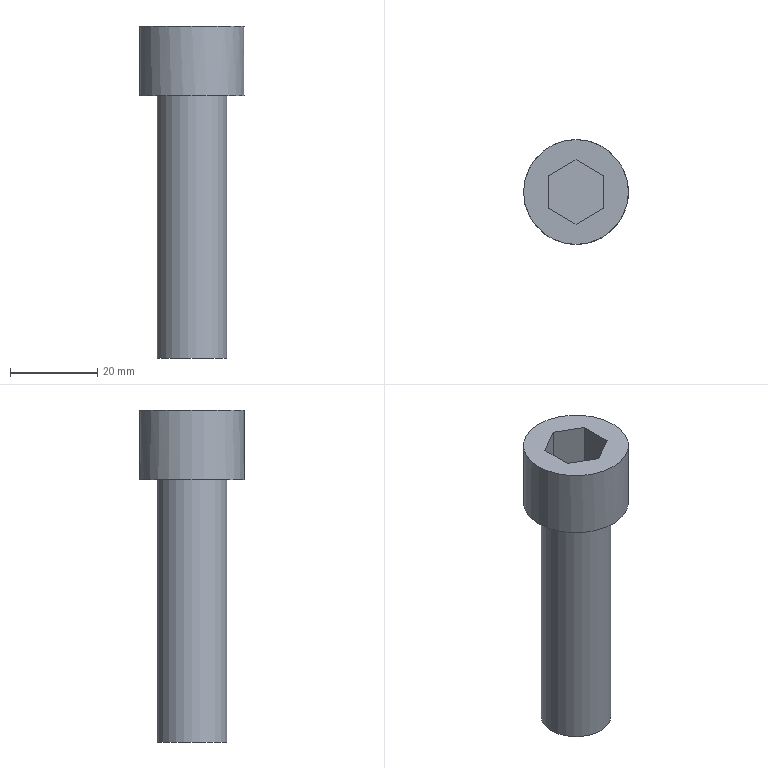Part | NX | features solid 2 | 1 solid | 12 faces | box 24 x 24 x 76 mm | volume 17940 mm3 | plane 10 | cylinder 2 | commonest cylinder face diameters 16 x1 24 x1
STEP:
#1=CARTESIAN_POINT('',(63.4,701.71,-169.));
#2=VERTEX_POINT('',#1);
#3=CARTESIAN_POINT('',(57.,698.015,-169.));
#4=VERTEX_POINT('',#3);
#5=CARTESIAN_POINT('',(60.2,699.862,-169.));
#6=DIRECTION('',(-0.866,-0.5,0.));
#7=VECTOR('',#6,1000.);
#8=LINE('',#5,#7);
#9=EDGE_CURVE('',#2,#4,#8,.T.);
#10=ORIENTED_EDGE('',*,*,#9,.T.);
#11=CARTESIAN_POINT('',(50.6,701.71,-169.));
#12=VERTEX_POINT('',#11);
#13=CARTESIAN_POINT('',(53.8,699.862,-169.));
#14=DIRECTION('',(-0.866,0.5,0.));
#15=VECTOR('',#14,1000.);
#16=LINE('',#13,#15);
#17=EDGE_CURVE('',#4,#12,#16,.T.);
#18=ORIENTED_EDGE('',*,*,#17,.T.);
#19=CARTESIAN_POINT('',(50.6,709.1,-169.));
#20=VERTEX_POINT('',#19);
#21=CARTESIAN_POINT('',(50.6,705.405,-169.));
#22=DIRECTION('',(0.,1.,0.));
#23=VECTOR('',#22,1000.);
#24=LINE('',#21,#23);
#25=EDGE_CURVE('',#12,#20,#24,.T.);
#26=ORIENTED_EDGE('',*,*,#25,.T.);
#27=CARTESIAN_POINT('',(57.,712.795,-169.));
#28=VERTEX_POINT('',#27);
#29=CARTESIAN_POINT('',(53.8,710.947,-169.));
#30=DIRECTION('',(0.866,0.5,0.));
#31=VECTOR('',#30,1000.);
#32=LINE('',#29,#31);
#33=EDGE_CURVE('',#20,#28,#32,.T.);
#34=ORIENTED_EDGE('',*,*,#33,.T.);
#35=CARTESIAN_POINT('',(63.4,709.1,-169.));
#36=VERTEX_POINT('',#35);
#37=CARTESIAN_POINT('',(60.2,710.947,-169.));
#38=DIRECTION('',(0.866,-0.5,0.));
#39=VECTOR('',#38,1000.);
#40=LINE('',#37,#39);
#41=EDGE_CURVE('',#28,#36,#40,.T.);
#42=ORIENTED_EDGE('',*,*,#41,.T.);
#43=CARTESIAN_POINT('',(63.4,705.405,-169.));
#44=DIRECTION('',(0.,-1.,0.));
#45=VECTOR('',#44,1000.);
#46=LINE('',#43,#45);
#47=EDGE_CURVE('',#36,#2,#46,.T.);
#48=ORIENTED_EDGE('',*,*,#47,.T.);
#49=EDGE_LOOP('',(#10,#18,#26,#34,#42,#48));
#50=FACE_BOUND('',#49,.T.);
#51=CARTESIAN_POINT('',(69.,705.405,-169.));
#52=VERTEX_POINT('',#51);
#53=CARTESIAN_POINT('',(57.,705.405,-169.));
#54=DIRECTION('',(0.,0.,1.));
#55=DIRECTION('',(1.,0.,0.));
#56=AXIS2_PLACEMENT_3D('',#53,#54,#55);
#57=CIRCLE('',#56,12.);
#58=EDGE_CURVE('',#52,#52,#57,.T.);
#59=ORIENTED_EDGE('',*,*,#58,.T.);
#60=EDGE_LOOP('',(#59));
#61=FACE_BOUND('',#60,.T.);
#62=CARTESIAN_POINT('',(57.,705.405,-169.));
#63=DIRECTION('',(0.,0.,1.));
#64=DIRECTION('',(-1.,0.,0.));
#65=AXIS2_PLACEMENT_3D('',#62,#63,#64);
#66=PLANE('',#65);
#67=ADVANCED_FACE('',(#50,#61),#66,.T.);
#68=CARTESIAN_POINT('',(65.,705.405,-185.));
#69=VERTEX_POINT('',#68);
#70=CARTESIAN_POINT('',(57.,705.405,-185.));
#71=DIRECTION('',(0.,0.,1.));
#72=DIRECTION('',(1.,0.,0.));
#73=AXIS2_PLACEMENT_3D('',#70,#71,#72);
#74=CIRCLE('',#73,8.);
#75=EDGE_CURVE('',#69,#69,#74,.T.);
#76=ORIENTED_EDGE('',*,*,#75,.T.);
#77=EDGE_LOOP('',(#76));
#78=FACE_BOUND('',#77,.T.);
#79=CARTESIAN_POINT('',(45.,705.405,-185.));
#80=VERTEX_POINT('',#79);
#81=CARTESIAN_POINT('',(57.,705.405,-185.));
#82=DIRECTION('',(0.,0.,-1.));
#83=DIRECTION('',(-1.,0.,0.));
#84=AXIS2_PLACEMENT_3D('',#81,#82,#83);
#85=CIRCLE('',#84,12.);
#86=EDGE_CURVE('',#80,#80,#85,.T.);
#87=ORIENTED_EDGE('',*,*,#86,.T.);
#88=EDGE_LOOP('',(#87));
#89=FACE_BOUND('',#88,.T.);
#90=CARTESIAN_POINT('',(57.,705.405,-185.));
#91=DIRECTION('',(0.,0.,-1.));
#92=DIRECTION('',(1.,0.,0.));
#93=AXIS2_PLACEMENT_3D('',#90,#91,#92);
#94=PLANE('',#93);
#95=ADVANCED_FACE('',(#78,#89),#94,.T.);
#96=ORIENTED_EDGE('',*,*,#58,.F.);
#97=EDGE_LOOP('',(#96));
#98=FACE_BOUND('',#97,.T.);
#99=ORIENTED_EDGE('',*,*,#86,.F.);
#100=EDGE_LOOP('',(#99));
#101=FACE_BOUND('',#100,.T.);
#102=CARTESIAN_POINT('',(57.,705.405,-185.));
#103=DIRECTION('',(0.,0.,1.));
#104=DIRECTION('',(-1.,0.,0.));
#105=AXIS2_PLACEMENT_3D('',#102,#103,#104);
#106=CYLINDRICAL_SURFACE('',#105,12.);
#107=ADVANCED_FACE('',(#98,#101),#106,.T.);
#108=ORIENTED_EDGE('',*,*,#9,.F.);
#109=CARTESIAN_POINT('',(63.4,701.71,-178.6));
#110=VERTEX_POINT('',#109);
#111=CARTESIAN_POINT('',(63.4,701.71,-178.6));
#112=DIRECTION('',(0.,0.,1.));
#113=VECTOR('',#112,1000.);
#114=LINE('',#111,#113);
#115=EDGE_CURVE('',#110,#2,#114,.T.);
#116=ORIENTED_EDGE('',*,*,#115,.F.);
#117=CARTESIAN_POINT('',(57.,698.015,-178.6));
#118=VERTEX_POINT('',#117);
#119=CARTESIAN_POINT('',(63.4,701.71,-178.6));
#120=DIRECTION('',(-0.866,-0.5,0.));
#121=VECTOR('',#120,1000.);
#122=LINE('',#119,#121);
#123=EDGE_CURVE('',#110,#118,#122,.T.);
#124=ORIENTED_EDGE('',*,*,#123,.T.);
#125=CARTESIAN_POINT('',(57.,698.015,-178.6));
#126=DIRECTION('',(0.,0.,1.));
#127=VECTOR('',#126,1000.);
#128=LINE('',#125,#127);
#129=EDGE_CURVE('',#118,#4,#128,.T.);
#130=ORIENTED_EDGE('',*,*,#129,.T.);
#131=EDGE_LOOP('',(#108,#116,#124,#130));
#132=FACE_BOUND('',#131,.T.);
#133=CARTESIAN_POINT('',(60.2,699.862,-170.6));
#134=DIRECTION('',(0.5,-0.866,0.));
#135=DIRECTION('',(-0.866,-0.5,0.));
#136=AXIS2_PLACEMENT_3D('',#133,#134,#135);
#137=PLANE('',#136);
#138=ADVANCED_FACE('',(#132),#137,.F.);
#139=ORIENTED_EDGE('',*,*,#47,.F.);
#140=CARTESIAN_POINT('',(63.4,709.1,-178.6));
#141=VERTEX_POINT('',#140);
#142=CARTESIAN_POINT('',(63.4,709.1,-178.6));
#143=DIRECTION('',(0.,0.,1.));
#144=VECTOR('',#143,1000.);
#145=LINE('',#142,#144);
#146=EDGE_CURVE('',#141,#36,#145,.T.);
#147=ORIENTED_EDGE('',*,*,#146,.F.);
#148=CARTESIAN_POINT('',(63.4,709.1,-178.6));
#149=DIRECTION('',(0.,-1.,0.));
#150=VECTOR('',#149,1000.);
#151=LINE('',#148,#150);
#152=EDGE_CURVE('',#141,#110,#151,.T.);
#153=ORIENTED_EDGE('',*,*,#152,.T.);
#154=ORIENTED_EDGE('',*,*,#115,.T.);
#155=EDGE_LOOP('',(#139,#147,#153,#154));
#156=FACE_BOUND('',#155,.T.);
#157=CARTESIAN_POINT('',(63.4,705.405,-170.6));
#158=DIRECTION('',(1.,0.,0.));
#159=DIRECTION('',(0.,0.,1.));
#160=AXIS2_PLACEMENT_3D('',#157,#158,#159);
#161=PLANE('',#160);
#162=ADVANCED_FACE('',(#156),#161,.F.);
#163=ORIENTED_EDGE('',*,*,#41,.F.);
#164=CARTESIAN_POINT('',(57.,712.795,-178.6));
#165=VERTEX_POINT('',#164);
#166=CARTESIAN_POINT('',(57.,712.795,-178.6));
#167=DIRECTION('',(0.,0.,1.));
#168=VECTOR('',#167,1000.);
#169=LINE('',#166,#168);
#170=EDGE_CURVE('',#165,#28,#169,.T.);
#171=ORIENTED_EDGE('',*,*,#170,.F.);
#172=CARTESIAN_POINT('',(57.,712.795,-178.6));
#173=DIRECTION('',(0.866,-0.5,0.));
#174=VECTOR('',#173,1000.);
#175=LINE('',#172,#174);
#176=EDGE_CURVE('',#165,#141,#175,.T.);
#177=ORIENTED_EDGE('',*,*,#176,.T.);
#178=ORIENTED_EDGE('',*,*,#146,.T.);
#179=EDGE_LOOP('',(#163,#171,#177,#178));
#180=FACE_BOUND('',#179,.T.);
#181=CARTESIAN_POINT('',(60.2,710.947,-170.6));
#182=DIRECTION('',(0.5,0.866,0.));
#183=DIRECTION('',(0.866,-0.5,0.));
#184=AXIS2_PLACEMENT_3D('',#181,#182,#183);
#185=PLANE('',#184);
#186=ADVANCED_FACE('',(#180),#185,.F.);
#187=ORIENTED_EDGE('',*,*,#33,.F.);
#188=CARTESIAN_POINT('',(50.6,709.1,-178.6));
#189=VERTEX_POINT('',#188);
#190=CARTESIAN_POINT('',(50.6,709.1,-178.6));
#191=DIRECTION('',(0.,0.,1.));
#192=VECTOR('',#191,1000.);
#193=LINE('',#190,#192);
#194=EDGE_CURVE('',#189,#20,#193,.T.);
#195=ORIENTED_EDGE('',*,*,#194,.F.);
#196=CARTESIAN_POINT('',(50.6,709.1,-178.6));
#197=DIRECTION('',(0.866,0.5,0.));
#198=VECTOR('',#197,1000.);
#199=LINE('',#196,#198);
#200=EDGE_CURVE('',#189,#165,#199,.T.);
#201=ORIENTED_EDGE('',*,*,#200,.T.);
#202=ORIENTED_EDGE('',*,*,#170,.T.);
#203=EDGE_LOOP('',(#187,#195,#201,#202));
#204=FACE_BOUND('',#203,.T.);
#205=CARTESIAN_POINT('',(53.8,710.947,-170.6));
#206=DIRECTION('',(-0.5,0.866,0.));
#207=DIRECTION('',(0.866,0.5,0.));
#208=AXIS2_PLACEMENT_3D('',#205,#206,#207);
#209=PLANE('',#208);
#210=ADVANCED_FACE('',(#204),#209,.F.);
#211=ORIENTED_EDGE('',*,*,#25,.F.);
#212=CARTESIAN_POINT('',(50.6,701.71,-178.6));
#213=VERTEX_POINT('',#212);
#214=CARTESIAN_POINT('',(50.6,701.71,-178.6));
#215=DIRECTION('',(0.,0.,1.));
#216=VECTOR('',#215,1000.);
#217=LINE('',#214,#216);
#218=EDGE_CURVE('',#213,#12,#217,.T.);
#219=ORIENTED_EDGE('',*,*,#218,.F.);
#220=CARTESIAN_POINT('',(50.6,701.71,-178.6));
#221=DIRECTION('',(0.,1.,0.));
#222=VECTOR('',#221,1000.);
#223=LINE('',#220,#222);
#224=EDGE_CURVE('',#213,#189,#223,.T.);
#225=ORIENTED_EDGE('',*,*,#224,.T.);
#226=ORIENTED_EDGE('',*,*,#194,.T.);
#227=EDGE_LOOP('',(#211,#219,#225,#226));
#228=FACE_BOUND('',#227,.T.);
#229=CARTESIAN_POINT('',(50.6,705.405,-170.6));
#230=DIRECTION('',(-1.,0.,0.));
#231=DIRECTION('',(0.,0.,-1.));
#232=AXIS2_PLACEMENT_3D('',#229,#230,#231);
#233=PLANE('',#232);
#234=ADVANCED_FACE('',(#228),#233,.F.);
#235=ORIENTED_EDGE('',*,*,#17,.F.);
#236=ORIENTED_EDGE('',*,*,#129,.F.);
#237=CARTESIAN_POINT('',(57.,698.015,-178.6));
#238=DIRECTION('',(-0.866,0.5,0.));
#239=VECTOR('',#238,1000.);
#240=LINE('',#237,#239);
#241=EDGE_CURVE('',#118,#213,#240,.T.);
#242=ORIENTED_EDGE('',*,*,#241,.T.);
#243=ORIENTED_EDGE('',*,*,#218,.T.);
#244=EDGE_LOOP('',(#235,#236,#242,#243));
#245=FACE_BOUND('',#244,.T.);
#246=CARTESIAN_POINT('',(53.8,699.862,-170.6));
#247=DIRECTION('',(-0.5,-0.866,0.));
#248=DIRECTION('',(-0.866,0.5,0.));
#249=AXIS2_PLACEMENT_3D('',#246,#247,#248);
#250=PLANE('',#249);
#251=ADVANCED_FACE('',(#245),#250,.F.);
#252=ORIENTED_EDGE('',*,*,#241,.F.);
#253=ORIENTED_EDGE('',*,*,#123,.F.);
#254=ORIENTED_EDGE('',*,*,#152,.F.);
#255=ORIENTED_EDGE('',*,*,#176,.F.);
#256=ORIENTED_EDGE('',*,*,#200,.F.);
#257=ORIENTED_EDGE('',*,*,#224,.F.);
#258=EDGE_LOOP('',(#252,#253,#254,#255,#256,#257));
#259=FACE_BOUND('',#258,.T.);
#260=CARTESIAN_POINT('',(57.,705.405,-178.6));
#261=DIRECTION('',(0.,0.,-1.));
#262=DIRECTION('',(1.,0.,0.));
#263=AXIS2_PLACEMENT_3D('',#260,#261,#262);
#264=PLANE('',#263);
#265=ADVANCED_FACE('',(#259),#264,.F.);
#266=CARTESIAN_POINT('',(49.,705.405,-245.));
#267=VERTEX_POINT('',#266);
#268=CARTESIAN_POINT('',(57.,705.405,-245.));
#269=DIRECTION('',(0.,0.,-1.));
#270=DIRECTION('',(-1.,0.,0.));
#271=AXIS2_PLACEMENT_3D('',#268,#269,#270);
#272=CIRCLE('',#271,8.);
#273=EDGE_CURVE('',#267,#267,#272,.T.);
#274=ORIENTED_EDGE('',*,*,#273,.T.);
#275=EDGE_LOOP('',(#274));
#276=FACE_BOUND('',#275,.T.);
#277=CARTESIAN_POINT('',(57.,705.405,-245.));
#278=DIRECTION('',(0.,0.,-1.));
#279=DIRECTION('',(1.,0.,0.));
#280=AXIS2_PLACEMENT_3D('',#277,#278,#279);
#281=PLANE('',#280);
#282=ADVANCED_FACE('',(#276),#281,.T.);
#283=ORIENTED_EDGE('',*,*,#273,.F.);
#284=EDGE_LOOP('',(#283));
#285=FACE_BOUND('',#284,.T.);
#286=ORIENTED_EDGE('',*,*,#75,.F.);
#287=EDGE_LOOP('',(#286));
#288=FACE_BOUND('',#287,.T.);
#289=CARTESIAN_POINT('',(57.,705.405,-185.));
#290=DIRECTION('',(0.,0.,-1.));
#291=DIRECTION('',(1.,0.,0.));
#292=AXIS2_PLACEMENT_3D('',#289,#290,#291);
#293=CYLINDRICAL_SURFACE('',#292,8.);
#294=ADVANCED_FACE('',(#285,#288),#293,.T.);
#295=CLOSED_SHELL('',(#67,#95,#107,#138,#162,#186,#210,#234,#251,#265,#282,#294));
#296=MANIFOLD_SOLID_BREP('',#295);
#297=(LENGTH_UNIT()NAMED_UNIT(*)SI_UNIT(.MILLI.,.METRE.));
#298=UNCERTAINTY_MEASURE_WITH_UNIT(LENGTH_MEASURE(0.00001),#297,'','');
#299=(NAMED_UNIT(*)PLANE_ANGLE_UNIT()SI_UNIT($,.RADIAN.));
#300=(NAMED_UNIT(*)SI_UNIT($,.STERADIAN.)SOLID_ANGLE_UNIT());
#301=(GEOMETRIC_REPRESENTATION_CONTEXT(3)GLOBAL_UNCERTAINTY_ASSIGNED_CONTEXT((#298))GLOBAL_UNIT_ASSIGNED_CONTEXT((#297,#299,#300))REPRESENTATION_CONTEXT('',''));
#302=ADVANCED_BREP_SHAPE_REPRESENTATION('',(#296),#301);